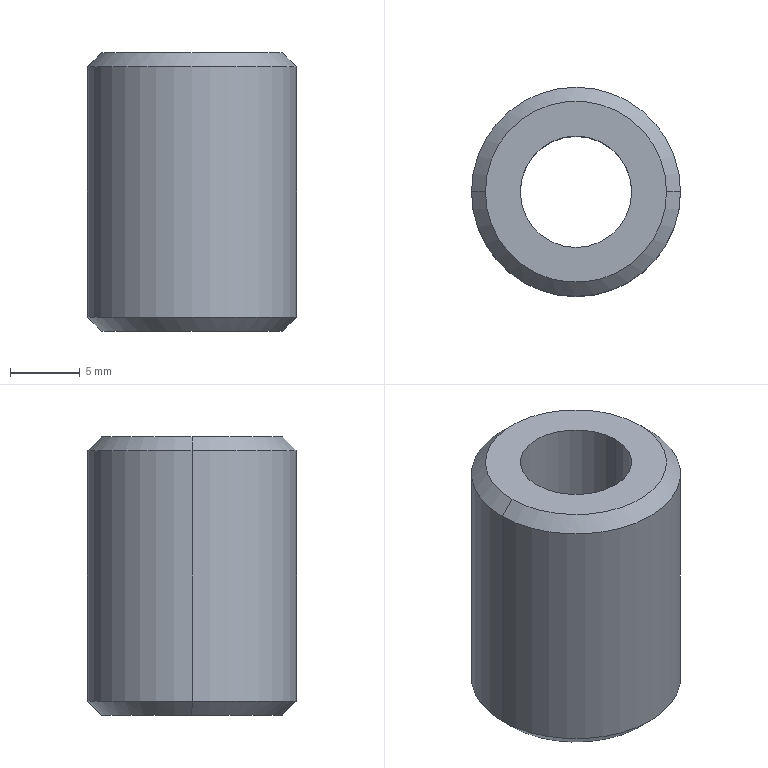Part | SolidWorks | features Chamfer 1, Extrusion 1, ICE 1 | 1 solid | 10 faces | box 15 x 15 x 20 mm | volume 2484 mm3 | cylinder 4 | cone 4 | plane 2 | commonest cylinder face diameters 8 x2 15 x2
STEP:
#1=CARTESIAN_POINT('',(-4.,0.,0.));
#2=VERTEX_POINT('',#1);
#3=CARTESIAN_POINT('',(4.,0.,0.));
#4=VERTEX_POINT('',#3);
#5=CARTESIAN_POINT('',(0.,0.,0.));
#6=DIRECTION('',(0.,0.,1.));
#7=DIRECTION('',(1.,0.,0.));
#8=AXIS2_PLACEMENT_3D('',#5,#6,#7);
#9=CIRCLE('',#8,4.);
#10=EDGE_CURVE('',#2,#4,#9,.T.);
#11=ORIENTED_EDGE('',*,*,#10,.F.);
#12=CARTESIAN_POINT('',(-4.,0.,20.));
#13=VERTEX_POINT('',#12);
#14=CARTESIAN_POINT('',(-4.,0.,0.));
#15=DIRECTION('',(0.,0.,1.));
#16=VECTOR('',#15,1000.);
#17=LINE('',#14,#16);
#18=EDGE_CURVE('',#2,#13,#17,.T.);
#19=ORIENTED_EDGE('',*,*,#18,.T.);
#20=CARTESIAN_POINT('',(4.,0.,20.));
#21=VERTEX_POINT('',#20);
#22=CARTESIAN_POINT('',(0.,0.,20.));
#23=DIRECTION('',(0.,0.,1.));
#24=DIRECTION('',(1.,0.,0.));
#25=AXIS2_PLACEMENT_3D('',#22,#23,#24);
#26=CIRCLE('',#25,4.);
#27=EDGE_CURVE('',#13,#21,#26,.T.);
#28=ORIENTED_EDGE('',*,*,#27,.T.);
#29=CARTESIAN_POINT('',(4.,0.,0.));
#30=DIRECTION('',(0.,0.,1.));
#31=VECTOR('',#30,1000.);
#32=LINE('',#29,#31);
#33=EDGE_CURVE('',#4,#21,#32,.T.);
#34=ORIENTED_EDGE('',*,*,#33,.F.);
#35=EDGE_LOOP('',(#11,#19,#28,#34));
#36=FACE_OUTER_BOUND('',#35,.T.);
#37=CARTESIAN_POINT('',(0.,0.,0.));
#38=DIRECTION('',(0.,0.,1.));
#39=DIRECTION('',(1.,0.,0.));
#40=AXIS2_PLACEMENT_3D('',#37,#38,#39);
#41=CYLINDRICAL_SURFACE('',#40,4.);
#42=ADVANCED_FACE('',(#36),#41,.F.);
#43=CARTESIAN_POINT('',(6.5,0.,20.));
#44=VERTEX_POINT('',#43);
#45=CARTESIAN_POINT('',(-6.5,0.,20.));
#46=VERTEX_POINT('',#45);
#47=CARTESIAN_POINT('',(0.,0.,20.));
#48=DIRECTION('',(0.,0.,1.));
#49=DIRECTION('',(1.,0.,0.));
#50=AXIS2_PLACEMENT_3D('',#47,#48,#49);
#51=CIRCLE('',#50,6.5);
#52=EDGE_CURVE('',#44,#46,#51,.T.);
#53=ORIENTED_EDGE('',*,*,#52,.F.);
#54=CARTESIAN_POINT('',(7.5,0.,19.));
#55=VERTEX_POINT('',#54);
#56=CARTESIAN_POINT('',(6.5,0.,20.));
#57=DIRECTION('',(0.7071,0.,-0.7071));
#58=VECTOR('',#57,1000.);
#59=LINE('',#56,#58);
#60=EDGE_CURVE('',#44,#55,#59,.T.);
#61=ORIENTED_EDGE('',*,*,#60,.T.);
#62=CARTESIAN_POINT('',(-7.5,0.,19.));
#63=VERTEX_POINT('',#62);
#64=CARTESIAN_POINT('',(0.,0.,19.));
#65=DIRECTION('',(0.,0.,-1.));
#66=DIRECTION('',(1.,0.,0.));
#67=AXIS2_PLACEMENT_3D('',#64,#65,#66);
#68=CIRCLE('',#67,7.5);
#69=EDGE_CURVE('',#63,#55,#68,.T.);
#70=ORIENTED_EDGE('',*,*,#69,.F.);
#71=CARTESIAN_POINT('',(-6.5,0.,20.));
#72=DIRECTION('',(-0.7071,0.,-0.7071));
#73=VECTOR('',#72,1000.);
#74=LINE('',#71,#73);
#75=EDGE_CURVE('',#46,#63,#74,.T.);
#76=ORIENTED_EDGE('',*,*,#75,.F.);
#77=EDGE_LOOP('',(#53,#61,#70,#76));
#78=FACE_OUTER_BOUND('',#77,.T.);
#79=CARTESIAN_POINT('',(0.,0.,20.));
#80=DIRECTION('',(0.,0.,-1.));
#81=DIRECTION('',(-1.,0.,0.));
#82=AXIS2_PLACEMENT_3D('',#79,#80,#81);
#83=CONICAL_SURFACE('',#82,6.5,0.7854);
#84=ADVANCED_FACE('',(#78),#83,.T.);
#85=CARTESIAN_POINT('',(-6.5,0.,0.));
#86=VERTEX_POINT('',#85);
#87=CARTESIAN_POINT('',(6.5,0.,0.));
#88=VERTEX_POINT('',#87);
#89=CARTESIAN_POINT('',(0.,0.,0.));
#90=DIRECTION('',(0.,0.,-1.));
#91=DIRECTION('',(1.,0.,0.));
#92=AXIS2_PLACEMENT_3D('',#89,#90,#91);
#93=CIRCLE('',#92,6.5);
#94=EDGE_CURVE('',#86,#88,#93,.T.);
#95=ORIENTED_EDGE('',*,*,#94,.F.);
#96=CARTESIAN_POINT('',(-7.5,0.,1.));
#97=VERTEX_POINT('',#96);
#98=CARTESIAN_POINT('',(-7.5,0.,1.));
#99=DIRECTION('',(-0.7071,0.,0.7071));
#100=VECTOR('',#99,1000.);
#101=LINE('',#98,#100);
#102=EDGE_CURVE('',#86,#97,#101,.T.);
#103=ORIENTED_EDGE('',*,*,#102,.T.);
#104=CARTESIAN_POINT('',(7.5,0.,1.));
#105=VERTEX_POINT('',#104);
#106=CARTESIAN_POINT('',(0.,0.,1.));
#107=DIRECTION('',(0.,0.,1.));
#108=DIRECTION('',(1.,0.,0.));
#109=AXIS2_PLACEMENT_3D('',#106,#107,#108);
#110=CIRCLE('',#109,7.5);
#111=EDGE_CURVE('',#105,#97,#110,.T.);
#112=ORIENTED_EDGE('',*,*,#111,.F.);
#113=CARTESIAN_POINT('',(7.5,0.,1.));
#114=DIRECTION('',(0.7071,0.,0.7071));
#115=VECTOR('',#114,1000.);
#116=LINE('',#113,#115);
#117=EDGE_CURVE('',#88,#105,#116,.T.);
#118=ORIENTED_EDGE('',*,*,#117,.F.);
#119=EDGE_LOOP('',(#95,#103,#112,#118));
#120=FACE_OUTER_BOUND('',#119,.T.);
#121=CARTESIAN_POINT('',(0.,0.,1.));
#122=DIRECTION('',(0.,0.,1.));
#123=DIRECTION('',(1.,0.,0.));
#124=AXIS2_PLACEMENT_3D('',#121,#122,#123);
#125=CONICAL_SURFACE('',#124,7.5,0.7854);
#126=ADVANCED_FACE('',(#120),#125,.T.);
#127=ORIENTED_EDGE('',*,*,#69,.T.);
#128=CARTESIAN_POINT('',(7.5,0.,20.));
#129=DIRECTION('',(0.,0.,-1.));
#130=VECTOR('',#129,1000.);
#131=LINE('',#128,#130);
#132=EDGE_CURVE('',#55,#105,#131,.T.);
#133=ORIENTED_EDGE('',*,*,#132,.T.);
#134=ORIENTED_EDGE('',*,*,#111,.T.);
#135=CARTESIAN_POINT('',(-7.5,0.,20.));
#136=DIRECTION('',(0.,0.,-1.));
#137=VECTOR('',#136,1000.);
#138=LINE('',#135,#137);
#139=EDGE_CURVE('',#63,#97,#138,.T.);
#140=ORIENTED_EDGE('',*,*,#139,.F.);
#141=EDGE_LOOP('',(#127,#133,#134,#140));
#142=FACE_OUTER_BOUND('',#141,.T.);
#143=CARTESIAN_POINT('',(0.,0.,20.));
#144=DIRECTION('',(0.,0.,-1.));
#145=DIRECTION('',(-1.,0.,0.));
#146=AXIS2_PLACEMENT_3D('',#143,#144,#145);
#147=CYLINDRICAL_SURFACE('',#146,7.5);
#148=ADVANCED_FACE('',(#142),#147,.T.);
#149=ORIENTED_EDGE('',*,*,#132,.F.);
#150=CARTESIAN_POINT('',(0.,0.,19.));
#151=DIRECTION('',(0.,0.,-1.));
#152=DIRECTION('',(1.,0.,0.));
#153=AXIS2_PLACEMENT_3D('',#150,#151,#152);
#154=CIRCLE('',#153,7.5);
#155=EDGE_CURVE('',#55,#63,#154,.T.);
#156=ORIENTED_EDGE('',*,*,#155,.T.);
#157=ORIENTED_EDGE('',*,*,#139,.T.);
#158=CARTESIAN_POINT('',(0.,0.,1.));
#159=DIRECTION('',(0.,0.,1.));
#160=DIRECTION('',(1.,0.,0.));
#161=AXIS2_PLACEMENT_3D('',#158,#159,#160);
#162=CIRCLE('',#161,7.5);
#163=EDGE_CURVE('',#97,#105,#162,.T.);
#164=ORIENTED_EDGE('',*,*,#163,.T.);
#165=EDGE_LOOP('',(#149,#156,#157,#164));
#166=FACE_OUTER_BOUND('',#165,.T.);
#167=CARTESIAN_POINT('',(0.,0.,20.));
#168=DIRECTION('',(0.,0.,-1.));
#169=DIRECTION('',(-1.,0.,0.));
#170=AXIS2_PLACEMENT_3D('',#167,#168,#169);
#171=CYLINDRICAL_SURFACE('',#170,7.5);
#172=ADVANCED_FACE('',(#166),#171,.T.);
#173=CARTESIAN_POINT('',(0.,0.,20.));
#174=DIRECTION('',(0.,0.,1.));
#175=DIRECTION('',(1.,0.,0.));
#176=AXIS2_PLACEMENT_3D('',#173,#174,#175);
#177=CIRCLE('',#176,4.);
#178=EDGE_CURVE('',#21,#13,#177,.T.);
#179=ORIENTED_EDGE('',*,*,#178,.F.);
#180=ORIENTED_EDGE('',*,*,#27,.F.);
#181=EDGE_LOOP('',(#179,#180));
#182=FACE_BOUND('',#181,.T.);
#183=CARTESIAN_POINT('',(0.,0.,20.));
#184=DIRECTION('',(0.,0.,1.));
#185=DIRECTION('',(1.,0.,0.));
#186=AXIS2_PLACEMENT_3D('',#183,#184,#185);
#187=CIRCLE('',#186,6.5);
#188=EDGE_CURVE('',#46,#44,#187,.T.);
#189=ORIENTED_EDGE('',*,*,#188,.T.);
#190=ORIENTED_EDGE('',*,*,#52,.T.);
#191=EDGE_LOOP('',(#189,#190));
#192=FACE_OUTER_BOUND('',#191,.T.);
#193=CARTESIAN_POINT('',(0.,0.,20.));
#194=DIRECTION('',(0.,0.,1.));
#195=DIRECTION('',(1.,0.,0.));
#196=AXIS2_PLACEMENT_3D('',#193,#194,#195);
#197=PLANE('',#196);
#198=ADVANCED_FACE('',(#182,#192),#197,.T.);
#199=CARTESIAN_POINT('',(0.,0.,0.));
#200=DIRECTION('',(0.,0.,1.));
#201=DIRECTION('',(1.,0.,0.));
#202=AXIS2_PLACEMENT_3D('',#199,#200,#201);
#203=CIRCLE('',#202,4.);
#204=EDGE_CURVE('',#4,#2,#203,.T.);
#205=ORIENTED_EDGE('',*,*,#204,.T.);
#206=ORIENTED_EDGE('',*,*,#10,.T.);
#207=EDGE_LOOP('',(#205,#206));
#208=FACE_BOUND('',#207,.T.);
#209=CARTESIAN_POINT('',(0.,0.,0.));
#210=DIRECTION('',(0.,0.,-1.));
#211=DIRECTION('',(1.,0.,0.));
#212=AXIS2_PLACEMENT_3D('',#209,#210,#211);
#213=CIRCLE('',#212,6.5);
#214=EDGE_CURVE('',#88,#86,#213,.T.);
#215=ORIENTED_EDGE('',*,*,#214,.T.);
#216=ORIENTED_EDGE('',*,*,#94,.T.);
#217=EDGE_LOOP('',(#215,#216));
#218=FACE_OUTER_BOUND('',#217,.T.);
#219=CARTESIAN_POINT('',(0.,0.,0.));
#220=DIRECTION('',(0.,0.,1.));
#221=DIRECTION('',(1.,0.,0.));
#222=AXIS2_PLACEMENT_3D('',#219,#220,#221);
#223=PLANE('',#222);
#224=ADVANCED_FACE('',(#208,#218),#223,.F.);
#225=ORIENTED_EDGE('',*,*,#102,.F.);
#226=ORIENTED_EDGE('',*,*,#214,.F.);
#227=ORIENTED_EDGE('',*,*,#117,.T.);
#228=ORIENTED_EDGE('',*,*,#163,.F.);
#229=EDGE_LOOP('',(#225,#226,#227,#228));
#230=FACE_OUTER_BOUND('',#229,.T.);
#231=CARTESIAN_POINT('',(0.,0.,1.));
#232=DIRECTION('',(0.,0.,1.));
#233=DIRECTION('',(1.,0.,0.));
#234=AXIS2_PLACEMENT_3D('',#231,#232,#233);
#235=CONICAL_SURFACE('',#234,7.5,0.7854);
#236=ADVANCED_FACE('',(#230),#235,.T.);
#237=ORIENTED_EDGE('',*,*,#60,.F.);
#238=ORIENTED_EDGE('',*,*,#188,.F.);
#239=ORIENTED_EDGE('',*,*,#75,.T.);
#240=ORIENTED_EDGE('',*,*,#155,.F.);
#241=EDGE_LOOP('',(#237,#238,#239,#240));
#242=FACE_OUTER_BOUND('',#241,.T.);
#243=CARTESIAN_POINT('',(0.,0.,20.));
#244=DIRECTION('',(0.,0.,-1.));
#245=DIRECTION('',(-1.,0.,0.));
#246=AXIS2_PLACEMENT_3D('',#243,#244,#245);
#247=CONICAL_SURFACE('',#246,6.5,0.7854);
#248=ADVANCED_FACE('',(#242),#247,.T.);
#249=ORIENTED_EDGE('',*,*,#18,.F.);
#250=ORIENTED_EDGE('',*,*,#204,.F.);
#251=ORIENTED_EDGE('',*,*,#33,.T.);
#252=ORIENTED_EDGE('',*,*,#178,.T.);
#253=EDGE_LOOP('',(#249,#250,#251,#252));
#254=FACE_OUTER_BOUND('',#253,.T.);
#255=CARTESIAN_POINT('',(0.,0.,0.));
#256=DIRECTION('',(0.,0.,1.));
#257=DIRECTION('',(1.,0.,0.));
#258=AXIS2_PLACEMENT_3D('',#255,#256,#257);
#259=CYLINDRICAL_SURFACE('',#258,4.);
#260=ADVANCED_FACE('',(#254),#259,.F.);
#261=CLOSED_SHELL('',(#42,#84,#126,#148,#172,#198,#224,#236,#248,#260));
#262=MANIFOLD_SOLID_BREP('',#261);
#263=CARTESIAN_POINT('',(0.,0.,0.));
#264=DIRECTION('',(0.,0.,1.));
#265=DIRECTION('',(1.,0.,0.));
#266=AXIS2_PLACEMENT_3D('',#263,#264,#265);
#267=(LENGTH_UNIT()NAMED_UNIT(*)SI_UNIT(.MILLI.,.METRE.));
#268=UNCERTAINTY_MEASURE_WITH_UNIT(LENGTH_MEASURE(0.00001),#267,'','');
#269=(NAMED_UNIT(*)PLANE_ANGLE_UNIT()SI_UNIT($,.RADIAN.));
#270=(NAMED_UNIT(*)SI_UNIT($,.STERADIAN.)SOLID_ANGLE_UNIT());
#271=(GEOMETRIC_REPRESENTATION_CONTEXT(3)GLOBAL_UNCERTAINTY_ASSIGNED_CONTEXT((#268))GLOBAL_UNIT_ASSIGNED_CONTEXT((#267,#269,#270))REPRESENTATION_CONTEXT('',''));
#272=ADVANCED_BREP_SHAPE_REPRESENTATION('',(#262,#266),#271);